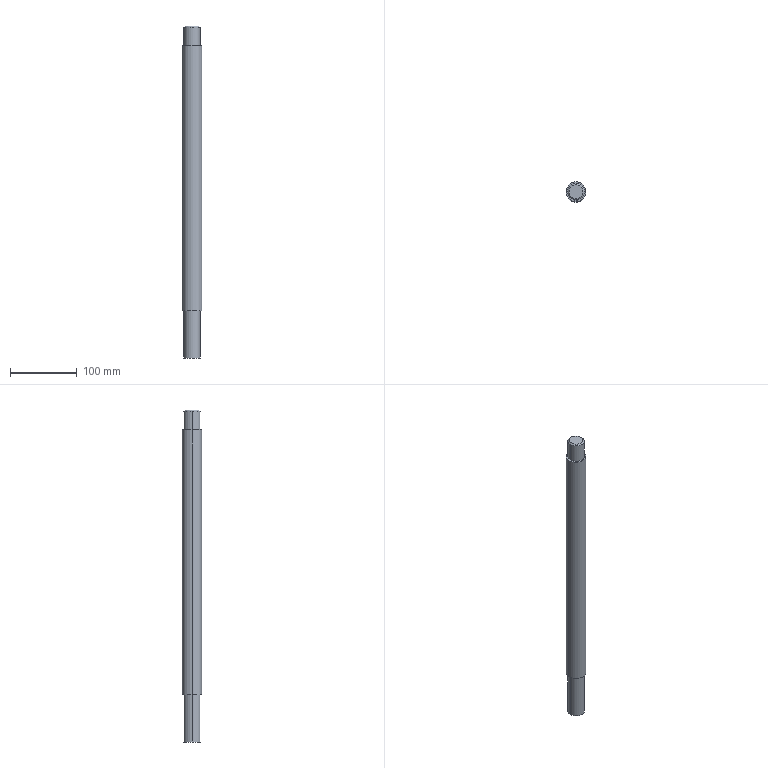Part | SolidWorks | features BaseBody 1 | 1 solid | 60 faces | box 30 x 30 x 499 mm | volume 328931 mm3 | cylinder 30 | plane 16 | torus 12 | cone 2 | commonest cylinder face diameters 1 x16 8 x8 25 x4 30 x2